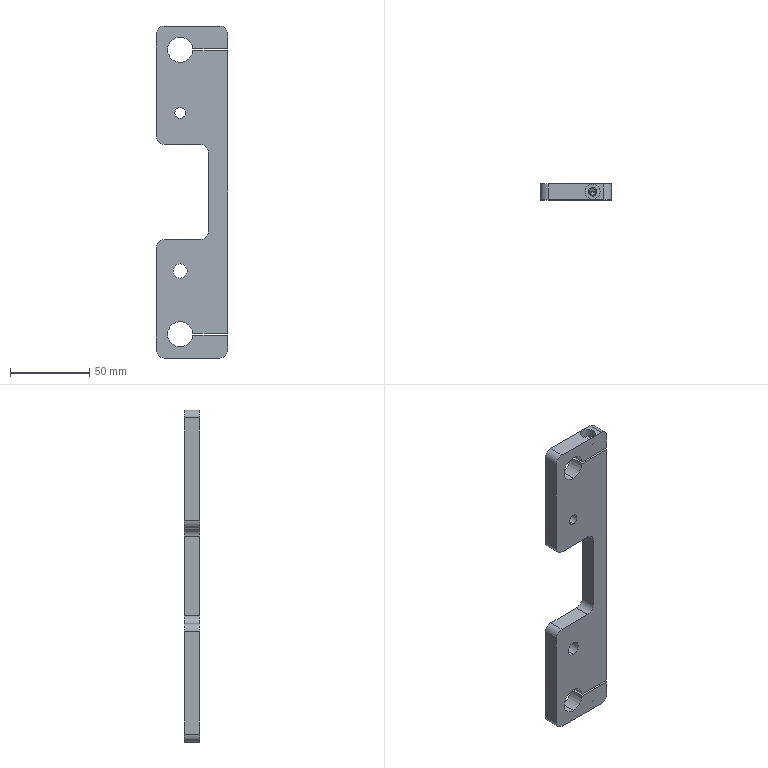Part | STEP file | PN_0034 | 1 solid | 52 faces | box 45 x 10 x 210 mm | volume 67263 mm3 | cylinder 30 | plane 18 | cone 4 | commonest cylinder face diameters 10 x8 16 x6 4.2 x4 5.5 x4 9.5 x4 6.8 x2